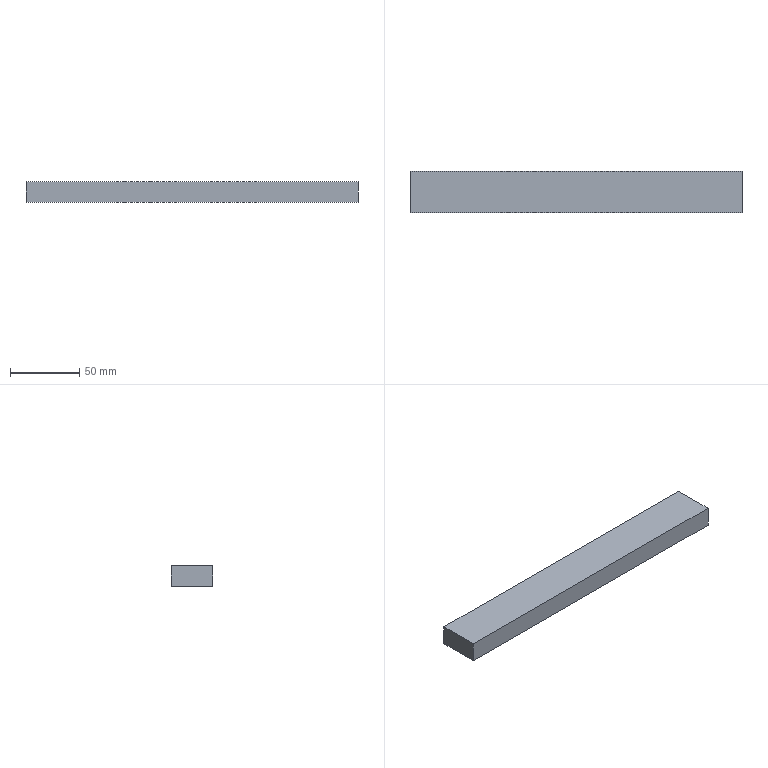Part | NX | features solid 2 | 1 solid | 6 faces | box 240 x 30 x 15 mm | volume 108000 mm3 | plane 6
STEP:
#1=CARTESIAN_POINT('',(-57.5,200.,-84.));
#2=VERTEX_POINT('',#1);
#3=CARTESIAN_POINT('',(-57.5,170.,-84.));
#4=VERTEX_POINT('',#3);
#5=CARTESIAN_POINT('',(-57.5,50.,-84.));
#6=DIRECTION('',(0.,-1.,0.));
#7=VECTOR('',#6,1000.);
#8=LINE('',#5,#7);
#9=EDGE_CURVE('',#2,#4,#8,.T.);
#10=ORIENTED_EDGE('',*,*,#9,.T.);
#11=CARTESIAN_POINT('',(-57.5,170.,-99.));
#12=VERTEX_POINT('',#11);
#13=CARTESIAN_POINT('',(-57.5,170.,-99.));
#14=DIRECTION('',(0.,0.,-1.));
#15=VECTOR('',#14,1000.);
#16=LINE('',#13,#15);
#17=EDGE_CURVE('',#12,#4,#16,.F.);
#18=ORIENTED_EDGE('',*,*,#17,.F.);
#19=CARTESIAN_POINT('',(-57.5,200.,-99.));
#20=VERTEX_POINT('',#19);
#21=CARTESIAN_POINT('',(-57.5,50.,-99.));
#22=DIRECTION('',(0.,1.,0.));
#23=VECTOR('',#22,1000.);
#24=LINE('',#21,#23);
#25=EDGE_CURVE('',#20,#12,#24,.F.);
#26=ORIENTED_EDGE('',*,*,#25,.F.);
#27=CARTESIAN_POINT('',(-57.5,200.,-99.));
#28=DIRECTION('',(0.,0.,-1.));
#29=VECTOR('',#28,1000.);
#30=LINE('',#27,#29);
#31=EDGE_CURVE('',#20,#2,#30,.F.);
#32=ORIENTED_EDGE('',*,*,#31,.T.);
#33=EDGE_LOOP('',(#10,#18,#26,#32));
#34=FACE_BOUND('',#33,.T.);
#35=CARTESIAN_POINT('',(-57.5,50.,-99.));
#36=DIRECTION('',(1.,0.,0.));
#37=DIRECTION('',(0.,0.,1.));
#38=AXIS2_PLACEMENT_3D('',#35,#36,#37);
#39=PLANE('',#38);
#40=ADVANCED_FACE('',(#34),#39,.T.);
#41=ORIENTED_EDGE('',*,*,#25,.T.);
#42=CARTESIAN_POINT('',(-297.5,170.,-99.));
#43=VERTEX_POINT('',#42);
#44=CARTESIAN_POINT('',(-47.5,170.,-99.));
#45=DIRECTION('',(-1.,0.,0.));
#46=VECTOR('',#45,1000.);
#47=LINE('',#44,#46);
#48=EDGE_CURVE('',#12,#43,#47,.T.);
#49=ORIENTED_EDGE('',*,*,#48,.T.);
#50=CARTESIAN_POINT('',(-297.5,200.,-99.));
#51=VERTEX_POINT('',#50);
#52=CARTESIAN_POINT('',(-297.5,300.,-99.));
#53=DIRECTION('',(0.,-1.,0.));
#54=VECTOR('',#53,1000.);
#55=LINE('',#52,#54);
#56=EDGE_CURVE('',#51,#43,#55,.T.);
#57=ORIENTED_EDGE('',*,*,#56,.F.);
#58=CARTESIAN_POINT('',(-47.5,200.,-99.));
#59=DIRECTION('',(-1.,0.,0.));
#60=VECTOR('',#59,1000.);
#61=LINE('',#58,#60);
#62=EDGE_CURVE('',#20,#51,#61,.T.);
#63=ORIENTED_EDGE('',*,*,#62,.F.);
#64=EDGE_LOOP('',(#41,#49,#57,#63));
#65=FACE_BOUND('',#64,.T.);
#66=CARTESIAN_POINT('',(-47.5,50.,-99.));
#67=DIRECTION('',(0.,0.,1.));
#68=DIRECTION('',(-1.,0.,0.));
#69=AXIS2_PLACEMENT_3D('',#66,#67,#68);
#70=PLANE('',#69);
#71=ADVANCED_FACE('',(#65),#70,.F.);
#72=ORIENTED_EDGE('',*,*,#56,.T.);
#73=CARTESIAN_POINT('',(-297.5,170.,-84.));
#74=VERTEX_POINT('',#73);
#75=CARTESIAN_POINT('',(-297.5,170.,-99.));
#76=DIRECTION('',(0.,0.,1.));
#77=VECTOR('',#76,1000.);
#78=LINE('',#75,#77);
#79=EDGE_CURVE('',#43,#74,#78,.T.);
#80=ORIENTED_EDGE('',*,*,#79,.T.);
#81=CARTESIAN_POINT('',(-297.5,200.,-84.));
#82=VERTEX_POINT('',#81);
#83=CARTESIAN_POINT('',(-297.5,50.,-84.));
#84=DIRECTION('',(0.,1.,0.));
#85=VECTOR('',#84,1000.);
#86=LINE('',#83,#85);
#87=EDGE_CURVE('',#82,#74,#86,.F.);
#88=ORIENTED_EDGE('',*,*,#87,.F.);
#89=CARTESIAN_POINT('',(-297.5,200.,-99.));
#90=DIRECTION('',(0.,0.,1.));
#91=VECTOR('',#90,1000.);
#92=LINE('',#89,#91);
#93=EDGE_CURVE('',#51,#82,#92,.T.);
#94=ORIENTED_EDGE('',*,*,#93,.F.);
#95=EDGE_LOOP('',(#72,#80,#88,#94));
#96=FACE_BOUND('',#95,.T.);
#97=CARTESIAN_POINT('',(-297.5,300.,-84.));
#98=DIRECTION('',(1.,0.,0.));
#99=DIRECTION('',(0.,1.,0.));
#100=AXIS2_PLACEMENT_3D('',#97,#98,#99);
#101=PLANE('',#100);
#102=ADVANCED_FACE('',(#96),#101,.F.);
#103=CARTESIAN_POINT('',(-47.5,200.,-84.));
#104=DIRECTION('',(1.,0.,0.));
#105=VECTOR('',#104,1000.);
#106=LINE('',#103,#105);
#107=EDGE_CURVE('',#2,#82,#106,.F.);
#108=ORIENTED_EDGE('',*,*,#107,.T.);
#109=ORIENTED_EDGE('',*,*,#87,.T.);
#110=CARTESIAN_POINT('',(-47.5,170.,-84.));
#111=DIRECTION('',(1.,0.,0.));
#112=VECTOR('',#111,1000.);
#113=LINE('',#110,#112);
#114=EDGE_CURVE('',#4,#74,#113,.F.);
#115=ORIENTED_EDGE('',*,*,#114,.F.);
#116=ORIENTED_EDGE('',*,*,#9,.F.);
#117=EDGE_LOOP('',(#108,#109,#115,#116));
#118=FACE_BOUND('',#117,.T.);
#119=CARTESIAN_POINT('',(-47.5,50.,-84.));
#120=DIRECTION('',(0.,0.,1.));
#121=DIRECTION('',(-1.,0.,0.));
#122=AXIS2_PLACEMENT_3D('',#119,#120,#121);
#123=PLANE('',#122);
#124=ADVANCED_FACE('',(#118),#123,.T.);
#125=ORIENTED_EDGE('',*,*,#79,.F.);
#126=ORIENTED_EDGE('',*,*,#48,.F.);
#127=ORIENTED_EDGE('',*,*,#17,.T.);
#128=ORIENTED_EDGE('',*,*,#114,.T.);
#129=EDGE_LOOP('',(#125,#126,#127,#128));
#130=FACE_BOUND('',#129,.T.);
#131=CARTESIAN_POINT('',(-47.5,170.,-99.));
#132=DIRECTION('',(0.,-1.,0.));
#133=DIRECTION('',(0.,0.,-1.));
#134=AXIS2_PLACEMENT_3D('',#131,#132,#133);
#135=PLANE('',#134);
#136=ADVANCED_FACE('',(#130),#135,.T.);
#137=ORIENTED_EDGE('',*,*,#93,.T.);
#138=ORIENTED_EDGE('',*,*,#107,.F.);
#139=ORIENTED_EDGE('',*,*,#31,.F.);
#140=ORIENTED_EDGE('',*,*,#62,.T.);
#141=EDGE_LOOP('',(#137,#138,#139,#140));
#142=FACE_BOUND('',#141,.T.);
#143=CARTESIAN_POINT('',(-47.5,200.,-99.));
#144=DIRECTION('',(0.,-1.,0.));
#145=DIRECTION('',(0.,0.,-1.));
#146=AXIS2_PLACEMENT_3D('',#143,#144,#145);
#147=PLANE('',#146);
#148=ADVANCED_FACE('',(#142),#147,.F.);
#149=CLOSED_SHELL('',(#40,#71,#102,#124,#136,#148));
#150=MANIFOLD_SOLID_BREP('',#149);
#151=(LENGTH_UNIT()NAMED_UNIT(*)SI_UNIT(.MILLI.,.METRE.));
#152=UNCERTAINTY_MEASURE_WITH_UNIT(LENGTH_MEASURE(0.00001),#151,'','');
#153=(NAMED_UNIT(*)PLANE_ANGLE_UNIT()SI_UNIT($,.RADIAN.));
#154=(NAMED_UNIT(*)SI_UNIT($,.STERADIAN.)SOLID_ANGLE_UNIT());
#155=(GEOMETRIC_REPRESENTATION_CONTEXT(3)GLOBAL_UNCERTAINTY_ASSIGNED_CONTEXT((#152))GLOBAL_UNIT_ASSIGNED_CONTEXT((#151,#153,#154))REPRESENTATION_CONTEXT('',''));
#156=ADVANCED_BREP_SHAPE_REPRESENTATION('',(#150),#155);